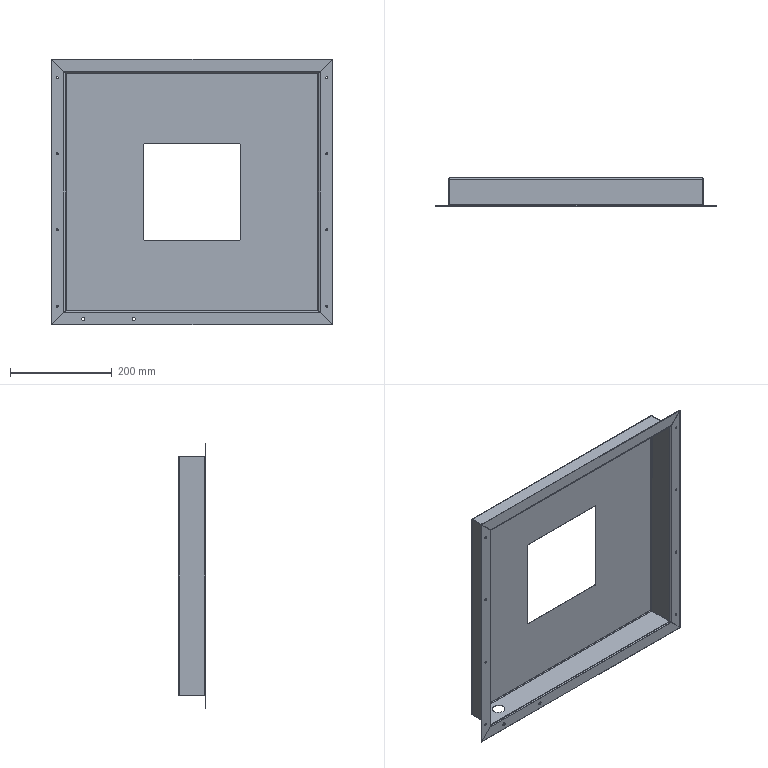Part | SolidWorks | features EdgeFlange 3, ICE 3, CornerFeat 2, Cut 1, Fillet 1, FlatPattern 1, SMBaseFlange 1, SheetMetal 1 | 1 solid | 124 faces | box 552.6 x 55 x 523.6 mm | volume 423620 mm3 | plane 74 | cylinder 42 | spline 8 | commonest cylinder face diameters 4 x16 3 x8 5.4 x8 6 x8 25 x2